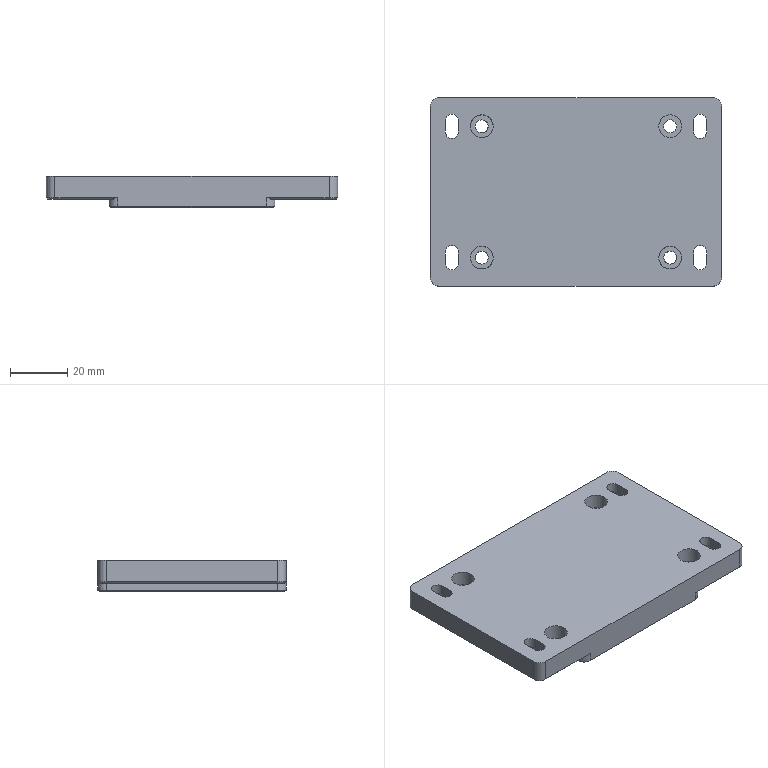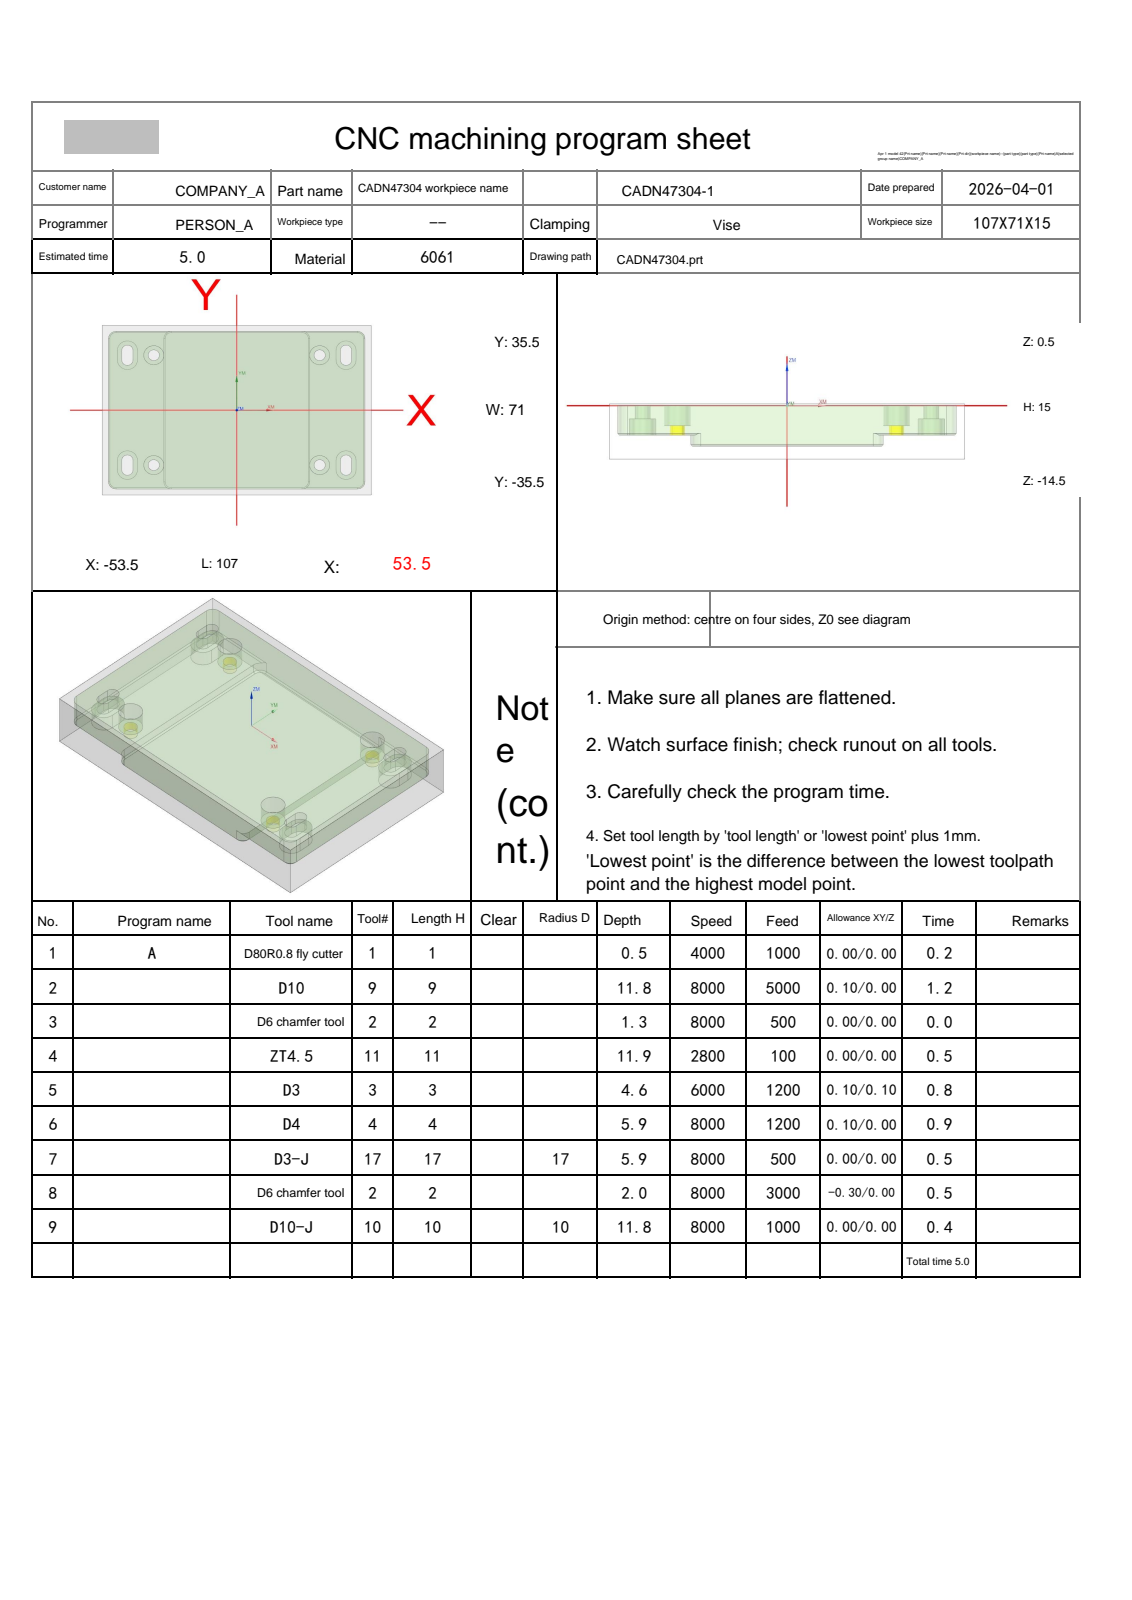NC program | NX | posted by the shop | part box 102 x 66 x 11 mm
Whole program:
%
O0001
(Machine time: 6.80 MIN)
(===Total Tool:8===)
(T1=D80R0.8 fly cutter D=80.  R=0.8  D-  H01 Z=-0.   )
(T9=D10     D=10.  R=0.   D-  H09 Z=-11.3 )
(T2=D6 chamfer tool   D=6.   R=0.   D-  H02 Z=-1.5  )
(T11=ZT4.5  D=4.5  DR_a=118 D-  H11 Z=-11.35)
(T3=D3      D=3.   R=0.   D-  H03 Z=-4.1  )
(T4=D4      D=4.   R=0.   D-  H04 Z=-5.4  )
(T17=D3-J   D=3.   R=0.   D17 H17 Z=-5.4  )
(T10=D10-J  D=10.  R=0.   D10 H10 Z=-11.3 )
G80 G90 G17 G49 G40
G91 G28 Z0
M01
N1 T01 M06
(D80R0.8 fly cutter  D=80. R=0.8 H=01 ce=0.00 di=0.00)
G00 G90 G54 X-96. Y0.0 M03 S4000
G43 H01 Z20.
M08
Z2.
G01 Z0.0 F1000.
X-91.
X91.
X96.
Z2.
G00 Z20.
G91 G28 Z0.0
M05
M09
G91 G28 Z0.0
M01
N2 T09 M06
(D10  D=10. R=0. H=09 ce=0.10 di=0.00)
G00 G90 G54 X0.0 Y38.1 M03 S8000
G43 H09 Z20.
M08
Z.5
G01 X48. Z.396 F5000.
G02 X56.1 Y30. Z.368 I0.0 J-8.1
G01 Y-30. Z.238
G02 X48. Y-38.1 Z.211 I-8.1 J0.0
G01 X-48. Z.003
G02 X-56.1 Y-30. Z-.025 I0.0 J8.1
G01 Y30. Z-.155
G02 X-48. Y38.1 Z-.183 I8.1 J0.0
G01 X48. Z-.391
G02 X56.1 Y30. Z-.418 I0.0 J-8.1
G01 Y-30. Z-.548
G02 X48. Y-38.1 Z-.576 I-8.1 J0.0
G01 X-48. Z-.784
G02 X-56.1 Y-30. Z-.812 I0.0 J8.1
G01 Y30. Z-.942
G02 X-48. Y38.1 Z-.969 I8.1 J0.0
G01 X48. Z-1.177
G02 X56.1 Y30. Z-1.205 I0.0 J-8.1
G01 Y-30. Z-1.335
G02 X48. Y-38.1 Z-1.363 I-8.1 J0.0
G01 X-48. Z-1.571
G02 X-56.1 Y-30. Z-1.598 I0.0 J8.1
G01 Y30. Z-1.728
G02 X-48. Y38.1 Z-1.756 I8.1 J0.0
G01 X48. Z-1.964
G02 X56.1 Y30. Z-1.992 I0.0 J-8.1
G01 Y-30. Z-2.122
G02 X48. Y-38.1 Z-2.149 I-8.1 J0.0
G01 X-48. Z-2.357
G02 X-56.1 Y-30. Z-2.385 I0.0 J8.1
G01 Y30. Z-2.515
G02 X-48. Y38.1 Z-2.543 I8.1 J0.0
G01 X48. Z-2.751
G02 X56.1 Y30. Z-2.778 I0.0 J-8.1
G01 Y-30. Z-2.908
G02 X48. Y-38.1 Z-2.936 I-8.1 J0.0
G01 X-48. Z-3.144
G02 X-56.1 Y-30. Z-3.172 I0.0 J8.1
G01 Y30. Z-3.302
G02 X-48. Y38.1 Z-3.329 I8.1 J0.0
G01 X48. Z-3.537
G02 X56.1 Y30. Z-3.565 I0.0 J-8.1
G01 Y-30. Z-3.695
G02 X48. Y-38.1 Z-3.723 I-8.1 J0.0
G01 X-48. Z-3.931
G02 X-56.1 Y-30. Z-3.958 I0.0 J8.1
G01 Y30. Z-4.088
G02 X-48. Y38.1 Z-4.116 I8.1 J0.0
G01 X48. Z-4.324
G02 X56.1 Y30. Z-4.352 I0.0 J-8.1
G01 Y-30. Z-4.482
G02 X48. Y-38.1 Z-4.509 I-8.1 J0.0
G01 X-48. Z-4.717
G02 X-56.1 Y-30. Z-4.745 I0.0 J8.1
G01 Y30. Z-4.875
G02 X-48. Y38.1 Z-4.903 I8.1 J0.0
G01 X48. Z-5.111
G02 X56.1 Y30. Z-5.138 I0.0 J-8.1
G01 Y-30. Z-5.268
G02 X48. Y-38.1 Z-5.296 I-8.1 J0.0
G01 X-48. Z-5.504
G02 X-56.1 Y-30. Z-5.532 I0.0 J8.1
G01 Y30. Z-5.662
G02 X-48. Y38.1 Z-5.689 I8.1 J0.0
G01 X48. Z-5.897
G02 X56.1 Y30. Z-5.925 I0.0 J-8.1
G01 Y-30. Z-6.055
G02 X48. Y-38.1 Z-6.083 I-8.1 J0.0
G01 X-48. Z-6.291
G02 X-56.1 Y-30. Z-6.318 I0.0 J8.1
G01 Y30. Z-6.448
G02 X-48. Y38.1 Z-6.476 I8.1 J0.0
G01 X48. Z-6.684
G02 X56.1 Y30. Z-6.712 I0.0 J-8.1
G01 Y-30. Z-6.842
G02 X48. Y-38.1 Z-6.869 I-8.1 J0.0
G01 X-48. Z-7.077
G02 X-56.1 Y-30. Z-7.105 I0.0 J8.1
G01 Y30. Z-7.235
G02 X-48. Y38.1 Z-7.263 I8.1 J0.0
G01 X48. Z-7.471
G02 X56.1 Y30. Z-7.498 I0.0 J-8.1
G01 Y-30. Z-7.628
G02 X48. Y-38.1 Z-7.656 I-8.1 J0.0
G01 X-48. Z-7.864
G02 X-56.1 Y-30. Z-7.892 I0.0 J8.1
G01 Y30. Z-8.022
G02 X-48. Y38.1 Z-8.049 I8.1 J0.0
G01 X48. Z-8.257
G02 X56.1 Y30. Z-8.285 I0.0 J-8.1
G01 Y-30. Z-8.415
G02 X48. Y-38.1 Z-8.443 I-8.1 J0.0
G01 X-48. Z-8.651
G02 X-56.1 Y-30. Z-8.678 I0.0 J8.1
G01 Y30. Z-8.808
G02 X-48. Y38.1 Z-8.836 I8.1 J0.0
G01 X48. Z-9.044
G02 X56.1 Y30. Z-9.072 I0.0 J-8.1
G01 Y-30. Z-9.202
G02 X48. Y-38.1 Z-9.229 I-8.1 J0.0
G01 X-48. Z-9.437
G02 X-56.1 Y-30. Z-9.465 I0.0 J8.1
G01 Y30. Z-9.595
G02 X-48. Y38.1 Z-9.623 I8.1 J0.0
G01 X48. Z-9.831
G02 X56.1 Y30. Z-9.858 I0.0 J-8.1
G01 Y-30. Z-9.988
G02 X48. Y-38.1 Z-10.016 I-8.1 J0.0
G01 X-48. Z-10.224
G02 X-56.1 Y-30. Z-10.252 I0.0 J8.1
G01 Y30. Z-10.382
G02 X-48. Y38.1 Z-10.409 I8.1 J0.0
G01 X48. Z-10.617
G02 X56.1 Y30. Z-10.645 I0.0 J-8.1
G01 Y-30. Z-10.775
G02 X48. Y-38.1 Z-10.803 I-8.1 J0.0
G01 X-48. Z-11.011
G02 X-56.1 Y-30. Z-11.038 I0.0 J8.1
G01 Y30. Z-11.168
G02 X-48. Y38.1 Z-11.196 I8.1 J0.0
G01 X0.0 Z-11.3
X48.
G02 X56.1 Y30. I0.0 J-8.1
G01 Y-30.
G02 X48. Y-38.1 I-8.1 J0.0
G01 X-48.
G02 X-56.1 Y-30. I0.0 J8.1
G01 Y30.
G02 X-48. Y38.1 I8.1 J0.0
G01 X0.0
X.5
Z-10.3
G00 Z20.
G91 G28 Z0.0
M05
M09
G91 G28 Z0.0
M01
N3 T02 M06
(D6 chamfer tool  D=6. R=0. H=02 ce=0.00 di=0.00)
G00 G90 G54 X-33. Y23. M03 S8000
G43 H02 Z20.
M08
G98 G81 X-33. Y23. Z-.8 R1. F500.
Y-23.
X33.
Y23.
G80
G00 Z20.
G91 G28 Z0.0
M05
M09
G91 G28 Z0.0
M01
N4 T11 M06
(ZT4.5 D=4.5 DR_a=118 H=11)
G00 G90 G54 X-33. Y23. M03 S2800
G43 H11 Z20.
M08
G98 G83 X-33. Y23. Z-11.352 R1. F100. Q2.
Y-23.
X33.
Y23.
G80
G00 Z20.
G91 G28 Z0.0
M05
M09
G91 G28 Z0.0
M01
N5 T03 M06
(D3  D=3. R=0. H=03 ce=0.10 di=0.10)
G00 G90 G54 X-44.15 Y-23. M03 S6000
G43 H03 Z20.
M08
Z.5
G01 Y-25. Z.46 F1200.
G03 X-43.5 Y-25.65 Z.439 I.65 J0.0
X-42.85 Y-25. Z.419 I0.0 J.65
G01 Y-21. Z.339
G03 X-43.5 Y-20.35 Z.318 I-.65 J0.0
X-44.015 Y-20.603 Z.307 I0.0 J-.65
X-44.15 Y-21. Z.298 I.515 J-.397
G01 Y-25. Z.218
G03 X-43.5 Y-25.65 Z.197 I.65 J0.0
X-42.85 Y-25. Z.177 I0.0 J.65
G01 Y-21. Z.097
G03 X-43.5 Y-20.35 Z.076 I-.65 J0.0
X-44.015 Y-20.603 Z.064 I0.0 J-.65
X-44.15 Y-21. Z.056 I.515 J-.397
G01 Y-25. Z-.024
G03 X-43.5 Y-25.65 Z-.045 I.65 J0.0
X-42.85 Y-25. Z-.065 I0.0 J.65
G01 Y-21. Z-.145
G03 X-43.5 Y-20.35 Z-.166 I-.65 J0.0
X-44.015 Y-20.603 Z-.178 I0.0 J-.65
X-44.15 Y-21. Z-.186 I.515 J-.397
G01 Y-25. Z-.266
G03 X-43.5 Y-25.65 Z-.287 I.65 J0.0
X-42.85 Y-25. Z-.307 I0.0 J.65
G01 Y-21. Z-.387
G03 X-43.5 Y-20.35 Z-.408 I-.65 J0.0
X-44.015 Y-20.603 Z-.42 I0.0 J-.65
X-44.15 Y-21. Z-.428 I.515 J-.397
G01 Y-25. Z-.508
G03 X-43.5 Y-25.65 Z-.529 I.65 J0.0
X-42.85 Y-25. Z-.549 I0.0 J.65
G01 Y-21. Z-.63
G03 X-43.5 Y-20.35 Z-.65 I-.65 J0.0
X-44.015 Y-20.603 Z-.662 I0.0 J-.65
X-44.15 Y-21. Z-.67 I.515 J-.397
G01 Y-25. Z-.751
G03 X-43.5 Y-25.65 Z-.771 I.65 J0.0
X-42.85 Y-25. Z-.792 I0.0 J.65
G01 Y-21. Z-.872
G03 X-43.5 Y-20.35 Z-.892 I-.65 J0.0
X-44.015 Y-20.603 Z-.904 I0.0 J-.65
X-44.15 Y-21. Z-.913 I.515 J-.397
G01 Y-25. Z-.993
G03 X-43.5 Y-25.65 Z-1.013 I.65 J0.0
X-42.85 Y-25. Z-1.034 I0.0 J.65
G01 Y-21. Z-1.114
G03 X-43.5 Y-20.35 Z-1.134 I-.65 J0.0
X-44.015 Y-20.603 Z-1.146 I0.0 J-.65
X-44.15 Y-21. Z-1.155 I.515 J-.397
G01 Y-25. Z-1.235
G03 X-43.5 Y-25.65 Z-1.255 I.65 J0.0
X-42.85 Y-25. Z-1.276 I0.0 J.65
G01 Y-21. Z-1.356
G03 X-43.5 Y-20.35 Z-1.376 I-.65 J0.0
X-44.015 Y-20.603 Z-1.388 I0.0 J-.65
X-44.15 Y-21. Z-1.397 I.515 J-.397
G01 Y-25. Z-1.477
G03 X-43.5 Y-25.65 Z-1.497 I.65 J0.0
X-42.85 Y-25. Z-1.518 I0.0 J.65
G01 Y-21. Z-1.598
G03 X-43.5 Y-20.35 Z-1.618 I-.65 J0.0
X-44.015 Y-20.603 Z-1.63 I0.0 J-.65
X-44.15 Y-21. Z-1.639 I.515 J-.397
G01 Y-25. Z-1.719
G03 X-43.5 Y-25.65 Z-1.739 I.65 J0.0
X-42.85 Y-25. Z-1.76 I0.0 J.65
G01 Y-21. Z-1.84
G03 X-43.5 Y-20.35 Z-1.861 I-.65 J0.0
X-44.015 Y-20.603 Z-1.872 I0.0 J-.65
X-44.15 Y-21. Z-1.881 I.515 J-.397
G01 Y-25. Z-1.961
G03 X-43.5 Y-25.65 Z-1.982 I.65 J0.0
X-42.85 Y-25. Z-2.002 I0.0 J.65
G01 Y-21. Z-2.082
G03 X-43.5 Y-20.35 Z-2.103 I-.65 J0.0
X-44.015 Y-20.603 Z-2.115 I0.0 J-.65
X-44.15 Y-21. Z-2.123 I.515 J-.397
G01 Y-25. Z-2.203
G03 X-43.5 Y-25.65 Z-2.224 I.65 J0.0
X-42.85 Y-25. Z-2.244 I0.0 J.65
G01 Y-21. Z-2.324
G03 X-43.5 Y-20.35 Z-2.345 I-.65 J0.0
X-44.015 Y-20.603 Z-2.357 I0.0 J-.65
X-44.15 Y-21. Z-2.365 I.515 J-.397
G01 Y-25. Z-2.445
G03 X-43.5 Y-25.65 Z-2.466 I.65 J0.0
X-42.85 Y-25. Z-2.486 I0.0 J.65
G01 Y-21. Z-2.566
G03 X-43.5 Y-20.35 Z-2.587 I-.65 J0.0
X-44.015 Y-20.603 Z-2.599 I0.0 J-.65
X-44.15 Y-21. Z-2.607 I.515 J-.397
G01 Y-25. Z-2.687
G03 X-43.5 Y-25.65 Z-2.708 I.65 J0.0
X-42.85 Y-25. Z-2.728 I0.0 J.65
G01 Y-21. Z-2.808
G03 X-43.5 Y-20.35 Z-2.829 I-.65 J0.0
X-44.015 Y-20.603 Z-2.841 I0.0 J-.65
X-44.15 Y-21. Z-2.849 I.515 J-.397
G01 Y-25. Z-2.93
G03 X-43.5 Y-25.65 Z-2.95 I.65 J0.0
X-42.85 Y-25. Z-2.97 I0.0 J.65
G01 Y-21. Z-3.051
G03 X-43.5 Y-20.35 Z-3.071 I-.65 J0.0
X-44.015 Y-20.603 Z-3.083 I0.0 J-.65
X-44.15 Y-21. Z-3.092 I.515 J-.397
G01 Y-25. Z-3.172
G03 X-43.5 Y-25.65 Z-3.192 I.65 J0.0
X-42.85 Y-25. Z-3.213 I0.0 J.65
G01 Y-21. Z-3.293
G03 X-43.5 Y-20.35 Z-3.313 I-.65 J0.0
X-44.015 Y-20.603 Z-3.325 I0.0 J-.65
X-44.15 Y-21. Z-3.334 I.515 J-.397
G01 Y-25. Z-3.414
G03 X-43.5 Y-25.65 Z-3.434 I.65 J0.0
X-42.85 Y-25. Z-3.455 I0.0 J.65
G01 Y-21. Z-3.535
G03 X-43.5 Y-20.35 Z-3.555 I-.65 J0.0
X-44.015 Y-20.603 Z-3.567 I0.0 J-.65
X-44.15 Y-21. Z-3.576 I.515 J-.397
G01 Y-25. Z-3.656
G03 X-43.5 Y-25.65 Z-3.676 I.65 J0.0
X-42.85 Y-25. Z-3.697 I0.0 J.65
G01 Y-21. Z-3.777
G03 X-43.5 Y-20.35 Z-3.797 I-.65 J0.0
X-44.015 Y-20.603 Z-3.809 I0.0 J-.65
X-44.15 Y-21. Z-3.818 I.515 J-.397
G01 Y-25. Z-3.898
G03 X-43.5 Y-25.65 Z-3.918 I.65 J0.0
X-42.85 Y-25. Z-3.939 I0.0 J.65
G01 Y-21. Z-4.019
G03 X-43.5 Y-20.35 Z-4.039 I-.65 J0.0
X-44.015 Y-20.603 Z-4.051 I0.0 J-.65
X-44.15 Y-21. Z-4.06 I.515 J-.397
G01 Y-23. Z-4.1
Y-25.
G03 X-43.5 Y-25.65 I.65 J0.0
X-42.85 Y-25. I0.0 J.65
G01 Y-21.
G03 X-43.5 Y-20.35 I-.65 J0.0
X-44.15 Y-21. I0.0 J-.65
G01 Y-23.
Y-23.5
Z-3.1
G00 Z20.
Y23.
Z.5
G01 Y21. Z.46
G03 X-43.5 Y20.35 Z.439 I.65 J0.0
X-42.85 Y21. Z.419 I0.0 J.65
G01 Y25. Z.339
G03 X-43.5 Y25.65 Z.318 I-.65 J0.0
X-44.15 Y25. Z.298 I0.0 J-.65
G01 Y21. Z.218
G03 X-43.5 Y20.35 Z.197 I.65 J0.0
X-42.85 Y21. Z.177 I0.0 J.65
G01 Y25. Z.097
G03 X-43.5 Y25.65 Z.076 I-.65 J0.0
X-44.15 Y25. Z.056 I0.0 J-.65
G01 Y21. Z-.024
G03 X-43.5 Y20.35 Z-.045 I.65 J0.0
X-42.85 Y21. Z-.065 I0.0 J.65
G01 Y25. Z-.145
G03 X-43.5 Y25.65 Z-.166 I-.65 J0.0
X-44.15 Y25. Z-.186 I0.0 J-.65
G01 Y21. Z-.266
G03 X-43.5 Y20.35 Z-.287 I.65 J0.0
X-42.85 Y21. Z-.307 I0.0 J.65
G01 Y25. Z-.387
G03 X-43.5 Y25.65 Z-.408 I-.65 J0.0
X-44.15 Y25. Z-.428 I0.0 J-.65
G01 Y21. Z-.508
G03 X-43.5 Y20.35 Z-.529 I.65 J0.0
X-42.85 Y21. Z-.549 I0.0 J.65
G01 Y25. Z-.63
G03 X-43.5 Y25.65 Z-.65 I-.65 J0.0
X-44.15 Y25. Z-.67 I0.0 J-.65
G01 Y21. Z-.751
G03 X-43.5 Y20.35 Z-.771 I.65 J0.0
X-42.85 Y21. Z-.792 I0.0 J.65
G01 Y25. Z-.872
G03 X-43.5 Y25.65 Z-.892 I-.65 J0.0
X-44.15 Y25. Z-.913 I0.0 J-.65
G01 Y21. Z-.993
G03 X-43.5 Y20.35 Z-1.013 I.65 J0.0
X-42.85 Y21. Z-1.034 I0.0 J.65
G01 Y25. Z-1.114
G03 X-43.5 Y25.65 Z-1.134 I-.65 J0.0
X-44.15 Y25. Z-1.155 I0.0 J-.65
G01 Y21. Z-1.235
G03 X-43.5 Y20.35 Z-1.255 I.65 J0.0
X-42.85 Y21. Z-1.276 I0.0 J.65
G01 Y25. Z-1.356
G03 X-43.5 Y25.65 Z-1.376 I-.65 J0.0
X-44.15 Y25. Z-1.397 I0.0 J-.65
G01 Y21. Z-1.477
G03 X-43.5 Y20.35 Z-1.497 I.65 J0.0
X-42.85 Y21. Z-1.518 I0.0 J.65
G01 Y25. Z-1.598
G03 X-43.5 Y25.65 Z-1.618 I-.65 J0.0
X-44.15 Y25. Z-1.639 I0.0 J-.65
G01 Y21. Z-1.719
G03 X-43.5 Y20.35 Z-1.739 I.65 J0.0
X-42.85 Y21. Z-1.76 I0.0 J.65
G01 Y25. Z-1.84
G03 X-43.5 Y25.65 Z-1.861 I-.65 J0.0
X-44.15 Y25. Z-1.881 I0.0 J-.65
G01 Y21. Z-1.961
G03 X-43.5 Y20.35 Z-1.982 I.65 J0.0
X-42.85 Y21. Z-2.002 I0.0 J.65
G01 Y25. Z-2.082
G03 X-43.5 Y25.65 Z-2.103 I-.65 J0.0
X-44.15 Y25. Z-2.123 I0.0 J-.65
G01 Y21. Z-2.203
G03 X-43.5 Y20.35 Z-2.224 I.65 J0.0
X-42.85 Y21. Z-2.244 I0.0 J.65
G01 Y25. Z-2.324
G03 X-43.5 Y25.65 Z-2.345 I-.65 J0.0
X-44.15 Y25. Z-2.365 I0.0 J-.65
G01 Y21. Z-2.445
G03 X-43.5 Y20.35 Z-2.466 I.65 J0.0
X-42.85 Y21. Z-2.486 I0.0 J.65
G01 Y25. Z-2.566
G03 X-43.5 Y25.65 Z-2.587 I-.65 J0.0
X-44.15 Y25. Z-2.607 I0.0 J-.65
G01 Y21. Z-2.687
G03 X-43.5 Y20.35 Z-2.708 I.65 J0.0
X-42.85 Y21. Z-2.728 I0.0 J.65
G01 Y25. Z-2.808
G03 X-43.5 Y25.65 Z-2.829 I-.65 J0.0
X-44.15 Y25. Z-2.849 I0.0 J-.65
G01 Y21. Z-2.93
G03 X-43.5 Y20.35 Z-2.95 I.65 J0.0
X-42.85 Y21. Z-2.97 I0.0 J.65
G01 Y25. Z-3.051
G03 X-43.5 Y25.65 Z-3.071 I-.65 J0.0
X-44.15 Y25. Z-3.092 I0.0 J-.65
G01 Y21. Z-3.172
G03 X-43.5 Y20.35 Z-3.192 I.65 J0.0
X-42.85 Y21. Z-3.213 I0.0 J.65
G01 Y25. Z-3.293
G03 X-43.5 Y25.65 Z-3.313 I-.65 J0.0
X-44.15 Y25. Z-3.334 I0.0 J-.65
G01 Y21. Z-3.414
G03 X-43.5 Y20.35 Z-3.434 I.65 J0.0
X-42.85 Y21. Z-3.455 I0.0 J.65
G01 Y25. Z-3.535
G03 X-43.5 Y25.65 Z-3.555 I-.65 J0.0
X-44.15 Y25. Z-3.576 I0.0 J-.65
G01 Y21. Z-3.656
G03 X-43.5 Y20.35 Z-3.676 I.65 J0.0
X-42.85 Y21. Z-3.697 I0.0 J.65
G01 Y25. Z-3.777
G03 X-43.5 Y25.65 Z-3.797 I-.65 J0.0
X-44.15 Y25. Z-3.818 I0.0 J-.65
G01 Y21. Z-3.898
G03 X-43.5 Y20.35 Z-3.918 I.65 J0.0
X-42.85 Y21. Z-3.939 I0.0 J.65
G01 Y25. Z-4.019
G03 X-43.5 Y25.65 Z-4.039 I-.65 J0.0
X-44.15 Y25. Z-4.06 I0.0 J-.65
G01 Y23. Z-4.1
Y21.
G03 X-43.5 Y20.35 I.65 J0.0
X-42.85 Y21. I0.0 J.65
G01 Y25.
G03 X-43.5 Y25.65 I-.65 J0.0
X-44.15 Y25. I0.0 J-.65
G01 Y23.
Y22.5
Z-3.1
G00 Z20.
X44.15 Y23.
Z.5
G01 Y25. Z.46
G03 X43.5 Y25.65 Z.439 I-.65 J0.0
X42.85 Y25. Z.419 I0.0 J-.65
G01 Y21. Z.339
G03 X43.5 Y20.35 Z.318 I.65 J0.0
X44.15 Y21. Z.298 I0.0 J.65
G01 Y25. Z.218
G03 X43.5 Y25.65 Z.197 I-.65 J0.0
X42.85 Y25. Z.177 I0.0 J-.65
G01 Y21. Z.097
G03 X43.5 Y20.35 Z.076 I.65 J0.0
X44.15 Y21. Z.056 I0.0 J.65
G01 Y25. Z-.024
G03 X43.5 Y25.65 Z-.045 I-.65 J0.0
X42.85 Y25. Z-.065 I0.0 J-.65
G01 Y21. Z-.145
G03 X43.5 Y20.35 Z-.166 I.65 J0.0
X44.15 Y21. Z-.186 I0.0 J.65
G01 Y25. Z-.266
G03 X43.5 Y25.65 Z-.287 I-.65 J0.0
X42.85 Y25. Z-.307 I0.0 J-.65
G01 Y21. Z-.387
G03 X43.5 Y20.35 Z-.408 I.65 J0.0
X44.15 Y21. Z-.428 I0.0 J.65
G01 Y25. Z-.508
G03 X43.5 Y25.65 Z-.529 I-.65 J0.0
X42.85 Y25. Z-.549 I0.0 J-.65
G01 Y21. Z-.63
G03 X43.5 Y20.35 Z-.65 I.65 J0.0
X44.15 Y21. Z-.67 I0.0 J.65
G01 Y25. Z-.751
G03 X43.5 Y25.65 Z-.771 I-.65 J0.0
X42.85 Y25. Z-.792 I0.0 J-.65
G01 Y21. Z-.872
G03 X43.5 Y20.35 Z-.892 I.65 J0.0
X44.15 Y21. Z-.913 I0.0 J.65
G01 Y25. Z-.993
G03 X43.5 Y25.65 Z-1.013 I-.65 J0.0
X42.85 Y25. Z-1.034 I0.0 J-.65
G01 Y21. Z-1.114
G03 X43.5 Y20.35 Z-1.134 I.65 J0.0
X44.15 Y21. Z-1.155 I0.0 J.65
G01 Y25. Z-1.235
G03 X43.5 Y25.65 Z-1.255 I-.65 J0.0
X42.85 Y25. Z-1.276 I0.0 J-.65
G01 Y21. Z-1.356
G03 X43.5 Y20.35 Z-1.376 I.65 J0.0
X44.15 Y21. Z-1.397 I0.0 J.65
G01 Y25. Z-1.477
G03 X43.5 Y25.65 Z-1.497 I-.65 J0.0
X42.85 Y25. Z-1.518 I0.0 J-.65
G01 Y21. Z-1.598
G03 X43.5 Y20.35 Z-1.618 I.65 J0.0
X44.15 Y21. Z-1.639 I0.0 J.65
G01 Y25. Z-1.719
G03 X43.5 Y25.65 Z-1.739 I-.65 J0.0
X42.85 Y25. Z-1.76 I0.0 J-.65
G01 Y21. Z-1.84
G03 X43.5 Y20.35 Z-1.861 I.65 J0.0
X44.15 Y21. Z-1.881 I0.0 J.65
G01 Y25. Z-1.961
G03 X43.5 Y25.65 Z-1.982 I-.65 J0.0
X42.85 Y25. Z-2.002 I0.0 J-.65
G01 Y21. Z-2.082
G03 X43.5 Y20.35 Z-2.103 I.65 J0.0
X44.15 Y21. Z-2.123 I0.0 J.65
G01 Y25. Z-2.203
G03 X43.5 Y25.65 Z-2.224 I-.65 J0.0
X42.85 Y25. Z-2.244 I0.0 J-.65
G01 Y21. Z-2.324
G03 X43.5 Y20.35 Z-2.345 I.65 J0.0
X44.15 Y21. Z-2.365 I0.0 J.65
G01 Y25. Z-2.445
G03 X43.5 Y25.65 Z-2.466 I-.65 J0.0
X42.85 Y25. Z-2.486 I0.0 J-.65
G01 Y21. Z-2.566
G03 X43.5 Y20.35 Z-2.587 I.65 J0.0
X44.15 Y21. Z-2.607 I0.0 J.65
G01 Y25. Z-2.687
G03 X43.5 Y25.65 Z-2.708 I-.65 J0.0
X42.85 Y25. Z-2.728 I0.0 J-.65
G01 Y21. Z-2.808
G03 X43.5 Y20.35 Z-2.829 I.65 J0.0
X44.15 Y21. Z-2.849 I0.0 J.65
G01 Y25. Z-2.93
G03 X43.5 Y25.65 Z-2.95 I-.65 J0.0
X42.85 Y25. Z-2.97 I0.0 J-.65
G01 Y21. Z-3.051
G03 X43.5 Y20.35 Z-3.071 I.65 J0.0
X44.15 Y21. Z-3.092 I0.0 J.65
G01 Y25. Z-3.172
G03 X43.5 Y25.65 Z-3.192 I-.65 J0.0
X42.85 Y25. Z-3.213 I0.0 J-.65
G01 Y21. Z-3.293
G03 X43.5 Y20.35 Z-3.313 I.65 J0.0
X44.15 Y21. Z-3.334 I0.0 J.65
G01 Y25. Z-3.414
G03 X43.5 Y25.65 Z-3.434 I-.65 J0.0
X42.85 Y25. Z-3.455 I0.0 J-.65
G01 Y21. Z-3.535
G03 X43.5 Y20.35 Z-3.555 I.65 J0.0
X44.15 Y21. Z-3.576 I0.0 J.65
G01 Y25. Z-3.656
G03 X43.5 Y25.65 Z-3.676 I-.65 J0.0
X42.85 Y25. Z-3.697 I0.0 J-.65
G01 Y21. Z-3.777
G03 X43.5 Y20.35 Z-3.797 I.65 J0.0
X44.15 Y21. Z-3.818 I0.0 J.65
G01 Y25. Z-3.898
G03 X43.5 Y25.65 Z-3.918 I-.65 J0.0
X42.85 Y25. Z-3.939 I0.0 J-.65
G01 Y21. Z-4.019
G03 X43.5 Y20.35 Z-4.039 I.65 J0.0
X44.15 Y21. Z-4.06 I0.0 J.65
G01 Y23. Z-4.1
Y25.
G03 X43.5 Y25.65 I-.65 J0.0
X42.85 Y25. I0.0 J-.65
G01 Y21.
G03 X43.5 Y20.35 I.65 J0.0
X44.15 Y21. I0.0 J.65
G01 Y23.
Y23.5
Z-3.1
G00 Z20.
Y-23.
Z.5
G01 Y-21. Z.46
G03 X43.5 Y-20.35 Z.439 I-.65 J0.0
X42.85 Y-21. Z.419 I0.0 J-.65
G01 Y-25. Z.339
G03 X43.5 Y-25.65 Z.318 I.65 J0.0
X44.15 Y-25. Z.298 I0.0 J.65
G01 Y-21. Z.218
G03 X43.5 Y-20.35 Z.197 I-.65 J0.0
X42.85 Y-21. Z.177 I0.0 J-.65
G01 Y-25. Z.097
G03 X43.5 Y-25.65 Z.076 I.65 J0.0
X44.15 Y-25. Z.056 I0.0 J.65
G01 Y-21. Z-.024
G03 X43.5 Y-20.35 Z-.045 I-.65 J0.0
X42.85 Y-21. Z-.065 I0.0 J-.65
G01 Y-25. Z-.145
G03 X43.5 Y-25.65 Z-.166 I.65 J0.0
X44.15 Y-25. Z-.186 I0.0 J.65
G01 Y-21. Z-.266
G03 X43.5 Y-20.35 Z-.287 I-.65 J0.0
X42.85 Y-21. Z-.307 I0.0 J-.65
G01 Y-25. Z-.387
G03 X43.5 Y-25.65 Z-.408 I.65 J0.0
X44.15 Y-25. Z-.428 I0.0 J.65
G01 Y-21. Z-.508
G03 X43.5 Y-20.35 Z-.529 I-.65 J0.0
X42.85 Y-21. Z-.549 I0.0 J-.65
G01 Y-25. Z-.63
G03 X43.5 Y-25.65 Z-.65 I.65 J0.0
X44.15 Y-25. Z-.67 I0.0 J.65
G01 Y-21. Z-.751
G03 X43.5 Y-20.35 Z-.771 I-.65 J0.0
X42.85 Y-21. Z-.792 I0.0 J-.65
G01 Y-25. Z-.872
G03 X43.5 Y-25.65 Z-.892 I.65 J0.0
X44.15 Y-25. Z-.913 I0.0 J.65
G01 Y-21. Z-.993
G03 X43.5 Y-20.35 Z-1.013 I-.65 J0.0
X42.85 Y-21. Z-1.034 I0.0 J-.65
G01 Y-25. Z-1.114
G03 X43.5 Y-25.65 Z-1.134 I.65 J0.0
X44.15 Y-25. Z-1.155 I0.0 J.65
G01 Y-21. Z-1.235
G03 X43.5 Y-20.35 Z-1.255 I-.65 J0.0
X42.85 Y-21. Z-1.276 I0.0 J-.65
G01 Y-25. Z-1.356
G03 X43.5 Y-25.65 Z-1.376 I.65 J0.0
X44.15 Y-25. Z-1.397 I0.0 J.65
G01 Y-21. Z-1.477
G03 X43.5 Y-20.35 Z-1.497 I-.65 J0.0
X42.85 Y-21. Z-1.518 I0.0 J-.65
G01 Y-25. Z-1.598
G03 X43.5 Y-25.65 Z-1.618 I.65 J0.0
X44.15 Y-25. Z-1.639 I0.0 J.65
G01 Y-21. Z-1.719
G03 X43.5 Y-20.35 Z-1.739 I-.65 J0.0
X42.85 Y-21. Z-1.76 I0.0 J-.65
G01 Y-25. Z-1.84
G03 X43.5 Y-25.65 Z-1.861 I.65 J0.0
X44.15 Y-25. Z-1.881 I0.0 J.65
G01 Y-21. Z-1.961
G03 X43.5 Y-20.35 Z-1.982 I-.65 J0.0
X42.85 Y-21. Z-2.002 I0.0 J-.65
G01 Y-25. Z-2.082
G03 X43.5 Y-25.65 Z-2.103 I.65 J0.0
X44.15 Y-25. Z-2.123 I0.0 J.65
G01 Y-21. Z-2.203
G03 X43.5 Y-20.35 Z-2.224 I-.65 J0.0
X42.85 Y-21. Z-2.244 I0.0 J-.65
G01 Y-25. Z-2.324
G03 X43.5 Y-25.65 Z-2.345 I.65 J0.0
X44.15 Y-25. Z-2.365 I0.0 J.65
G01 Y-21. Z-2.445
G03 X43.5 Y-20.35 Z-2.466 I-.65 J0.0
X42.85 Y-21. Z-2.486 I0.0 J-.65
G01 Y-25. Z-2.566
G03 X43.5 Y-25.65 Z-2.587 I.65 J0.0
X44.15 Y-25. Z-2.607 I0.0 J.65
G01 Y-21. Z-2.687
G03 X43.5 Y-20.35 Z-2.708 I-.65 J0.0
X42.85 Y-21. Z-2.728 I0.0 J-.65
G01 Y-25. Z-2.808
G03 X43.5 Y-25.65 Z-2.829 I.65 J0.0
X44.15 Y-25. Z-2.849 I0.0 J.65
G01 Y-21. Z-2.93
G03 X43.5 Y-20.35 Z-2.95 I-.65 J0.0
X42.85 Y-21. Z-2.97 I0.0 J-.65
G01 Y-25. Z-3.051
G03 X43.5 Y-25.65 Z-3.071 I.65 J0.0
X44.15 Y-25. Z-3.092 I0.0 J.65
G01 Y-21. Z-3.172
G03 X43.5 Y-20.35 Z-3.192 I-.65 J0.0
X42.85 Y-21. Z-3.213 I0.0 J-.65
G01 Y-25. Z-3.293
G03 X43.5 Y-25.65 Z-3.313 I.65 J0.0
X44.15 Y-25. Z-3.334 I0.0 J.65
G01 Y-21. Z-3.414
G03 X43.5 Y-20.35 Z-3.434 I-.65 J0.0
X42.85 Y-21. Z-3.455 I0.0 J-.65
G01 Y-25. Z-3.535
G03 X43.5 Y-25.65 Z-3.555 I.65 J0.0
X44.15 Y-25. Z-3.576 I0.0 J.65
G01 Y-21. Z-3.656
G03 X43.5 Y-20.35 Z-3.676 I-.65 J0.0
X42.85 Y-21. Z-3.697 I0.0 J-.65
G01 Y-25. Z-3.777
G03 X43.5 Y-25.65 Z-3.797 I.65 J0.0
X44.15 Y-25. Z-3.818 I0.0 J.65
G01 Y-21. Z-3.898
G03 X43.5 Y-20.35 Z-3.918 I-.65 J0.0
X42.85 Y-21. Z-3.939 I0.0 J-.65
G01 Y-25. Z-4.019
G03 X43.5 Y-25.65 Z-4.039 I.65 J0.0
X44.15 Y-25. Z-4.06 I0.0 J.65
G01 Y-23. Z-4.1
Y-21.
G03 X43.5 Y-20.35 I-.65 J0.0
X42.85 Y-21. I0.0 J-.65
G01 Y-25.
G03 X43.5 Y-25.65 I.65 J0.0
X44.15 Y-25. I0.0 J.65
G01 Y-23.
Y-22.5
Z-3.1
G00 Z20.
G91 G28 Z0.0
M05
M09
G91 G28 Z0.0
M01
N6 T04 M06
(D4  D=4. R=0. H=04 ce=0.10 di=0.00)
G00 G90 G54 X-33. Y23. M03 S8000
G43 H04 Z20.
M08
Z.5
G03 X-32.05 Y22.05 I.95 J0.0 F1200.
X-31.1 Y23. I0.0 J.95
X-31.1 Y23. Z.2 I-1.9 J0.0
X-31.1 Y23. Z-.1 I-1.9 J0.0
X-31.1 Y23. Z-.4 I-1.9 J0.0
X-31.1 Y23. Z-.7 I-1.9 J0.0
X-31.1 Y23. Z-1. I-1.9 J0.0
X-31.1 Y23. Z-1.3 I-1.9 J0.0
X-31.1 Y23. Z-1.6 I-1.9 J0.0
X-31.1 Y23. Z-1.9 I-1.9 J0.0
X-31.1 Y23. Z-2.2 I-1.9 J0.0
X-31.1 Y23. Z-2.5 I-1.9 J0.0
X-31.1 Y23. Z-2.8 I-1.9 J0.0
X-31.1 Y23. Z-3.1 I-1.9 J0.0
X-31.1 Y23. Z-3.4 I-1.9 J0.0
X-31.1 Y23. Z-3.7 I-1.9 J0.0
X-31.1 Y23. Z-4. I-1.9 J0.0
X-31.1 Y23. Z-4.3 I-1.9 J0.0
X-31.1 Y23. Z-4.6 I-1.9 J0.0
X-31.1 Y23. Z-4.9 I-1.9 J0.0
X-31.1 Y23. Z-5.2 I-1.9 J0.0
X-33.95 Y21.355 Z-5.4 I-1.9 J0.0
X-33. Y21.1 I.95 J1.645
X-31.1 Y23. I0.0 J1.9
X-33. Y24.9 I-1.9 J0.0
X-34.9 Y23. I0.0 J-1.9
X-33.95 Y21.355 I1.9 J0.0
X-33.475 Y21.227 I.475 J.823
X-32.525 Y22.177 I0.0 J.95
X-33. Y23. I-.95 J0.0
G00 Z20.
Y-23.
Z.5
G03 X-32.05 Y-23.95 I.95 J0.0
X-31.1 Y-23. I0.0 J.95
X-31.1 Y-23. Z.2 I-1.9 J0.0
X-31.1 Y-23. Z-.1 I-1.9 J0.0
X-31.1 Y-23. Z-.4 I-1.9 J0.0
X-31.1 Y-23. Z-.7 I-1.9 J0.0
X-31.1 Y-23. Z-1. I-1.9 J0.0
X-31.1 Y-23. Z-1.3 I-1.9 J0.0
X-31.1 Y-23. Z-1.6 I-1.9 J0.0
X-31.1 Y-23. Z-1.9 I-1.9 J0.0
X-31.1 Y-23. Z-2.2 I-1.9 J0.0
X-31.1 Y-23. Z-2.5 I-1.9 J0.0
X-31.1 Y-23. Z-2.8 I-1.9 J0.0
X-31.1 Y-23. Z-3.1 I-1.9 J0.0
X-31.1 Y-23. Z-3.4 I-1.9 J0.0
X-31.1 Y-23. Z-3.7 I-1.9 J0.0
X-31.1 Y-23. Z-4. I-1.9 J0.0
X-31.1 Y-23. Z-4.3 I-1.9 J0.0
X-31.1 Y-23. Z-4.6 I-1.9 J0.0
X-31.1 Y-23. Z-4.9 I-1.9 J0.0
X-31.1 Y-23. Z-5.2 I-1.9 J0.0
X-33.95 Y-24.645 Z-5.4 I-1.9 J0.0
X-33. Y-24.9 I.95 J1.645
X-31.1 Y-23. I0.0 J1.9
X-33. Y-21.1 I-1.9 J0.0
X-34.9 Y-23. I0.0 J-1.9
X-33.95 Y-24.645 I1.9 J0.0
X-33.475 Y-24.773 I.475 J.823
X-32.525 Y-23.823 I0.0 J.95
X-33. Y-23. I-.95 J0.0
G00 Z20.
X33.
Z.5
G03 X33.95 Y-23.95 I.95 J0.0
X34.9 Y-23. I0.0 J.95
X34.9 Y-23. Z.2 I-1.9 J0.0
X34.9 Y-23. Z-.1 I-1.9 J0.0
X34.9 Y-23. Z-.4 I-1.9 J0.0
X34.9 Y-23. Z-.7 I-1.9 J0.0
X34.9 Y-23. Z-1. I-1.9 J0.0
X34.9 Y-23. Z-1.3 I-1.9 J0.0
X34.9 Y-23. Z-1.6 I-1.9 J0.0
X34.9 Y-23. Z-1.9 I-1.9 J0.0
X34.9 Y-23. Z-2.2 I-1.9 J0.0
X34.9 Y-23. Z-2.5 I-1.9 J0.0
X34.9 Y-23. Z-2.8 I-1.9 J0.0
X34.9 Y-23. Z-3.1 I-1.9 J0.0
X34.9 Y-23. Z-3.4 I-1.9 J0.0
X34.9 Y-23. Z-3.7 I-1.9 J0.0
X34.9 Y-23. Z-4. I-1.9 J0.0
X34.9 Y-23. Z-4.3 I-1.9 J0.0
X34.9 Y-23. Z-4.6 I-1.9 J0.0
X34.9 Y-23. Z-4.9 I-1.9 J0.0
X34.9 Y-23. Z-5.2 I-1.9 J0.0
X32.05 Y-24.645 Z-5.4 I-1.9 J0.0
X33. Y-24.9 I.95 J1.645
X34.9 Y-23. I0.0 J1.9
X33. Y-21.1 I-1.9 J0.0
X31.1 Y-23. I0.0 J-1.9
X32.05 Y-24.645 I1.9 J0.0
X32.525 Y-24.773 I.475 J.823
X33.475 Y-23.823 I0.0 J.95
X33. Y-23. I-.95 J0.0
G00 Z20.
Y23.
Z.5
G03 X33.95 Y22.05 I.95 J0.0
X34.9 Y23. I0.0 J.95
X34.9 Y23. Z.2 I-1.9 J0.0
X34.9 Y23. Z-.1 I-1.9 J0.0
X34.9 Y23. Z-.4 I-1.9 J0.0
X34.9 Y23. Z-.7 I-1.9 J0.0
X34.9 Y23. Z-1. I-1.9 J0.0
X34.9 Y23. Z-1.3 I-1.9 J0.0
X34.9 Y23. Z-1.6 I-1.9 J0.0
X34.9 Y23. Z-1.9 I-1.9 J0.0
X34.9 Y23. Z-2.2 I-1.9 J0.0
X34.9 Y23. Z-2.5 I-1.9 J0.0
X34.9 Y23. Z-2.8 I-1.9 J0.0
X34.9 Y23. Z-3.1 I-1.9 J0.0
X34.9 Y23. Z-3.4 I-1.9 J0.0
X34.9 Y23. Z-3.7 I-1.9 J0.0
X34.9 Y23. Z-4. I-1.9 J0.0
X34.9 Y23. Z-4.3 I-1.9 J0.0
X34.9 Y23. Z-4.6 I-1.9 J0.0
X34.9 Y23. Z-4.9 I-1.9 J0.0
X34.9 Y23. Z-5.2 I-1.9 J0.0
X32.05 Y21.355 Z-5.4 I-1.9 J0.0
X33. Y21.1 I.95 J1.645
X34.9 Y23. I0.0 J1.9
X33. Y24.9 I-1.9 J0.0
X31.1 Y23. I0.0 J-1.9
X32.05 Y21.355 I1.9 J0.0
X32.525 Y21.227 I.475 J.823
X33.475 Y22.177 I0.0 J.95
X33. Y23. I-.95 J0.0
G00 Z20.
G91 G28 Z0.0
M05
M09
G91 G28 Z0.0
M01
N7 T17 M06
(D3-J  D=3. R=0. H=17 ce=0.00 di=0.00)
G00 G90 G54 X-44. Y-22.8 M03 S6000
G43 H17 Z20.
M08
Z-3.4
G01 Z-3.9 F500.
G41 D17
X-44.05
G03 X-44.25 Y-23. I0.0 J-.2
G01 Y-25.
G03 X-43.5 Y-25.75 I.75 J0.0
X-42.75 Y-25. I0.0 J.75
G01 Y-21.
G03 X-43.5 Y-20.25 I-.75 J0.0
X-44.25 Y-21. I0.0 J-.75
G01 Y-23.
Y-23.5
G03 X-44.05 Y-23.7 I.2 J0.0
G01 G40 X-44.
Z-3.4
G00 Z20.
Y23.2
Z-3.4
G01 Z-3.9
G41 D17
X-44.05
G03 X-44.25 Y23. I0.0 J-.2
G01 Y21.
G03 X-43.5 Y20.25 I.75 J0.0
X-42.75 Y21. I0.0 J.75
G01 Y25.
G03 X-43.5 Y25.75 I-.75 J0.0
X-44.25 Y25. I0.0 J-.75
G01 Y23.
Y22.5
G03 X-44.05 Y22.3 I.2 J0.0
G01 G40 X-44.
Z-3.4
G00 Z20.
X44. Y22.8
Z-3.4
G01 Z-3.9
G41 D17
X44.05
G03 X44.25 Y23. I0.0 J.2
G01 Y25.
G03 X43.5 Y25.75 I-.75 J0.0
X42.75 Y25. I0.0 J-.75
G01 Y21.
G03 X43.5 Y20.25 I.75 J0.0
X44.25 Y21. I0.0 J.75
G01 Y23.
Y23.5
G03 X44.05 Y23.7 I-.2 J0.0
G01 G40 X44.
Z-3.4
G00 Z20.
Y-23.2
Z-3.4
G01 Z-3.9
G41 D17
X44.05
G03 X44.25 Y-23. I0.0 J.2
G01 Y-21.
G03 X43.5 Y-20.25 I-.75 J0.0
X42.75 Y-21. I0.0 J-.75
G01 Y-25.
G03 X43.5 Y-25.75 I.75 J0.0
X44.25 Y-25. I0.0 J.75
G01 Y-23.
Y-22.5
G03 X44.05 Y-22.3 I-.2 J0.0
G01 G40 X44.
Z-3.4
G00 Z20.
G00 G90 X-33. Y23. M03 S8000
Z20.
Z.5
G41 D17
G01 X-32.968 Y22.803 F500.
G03 X-31.742 Y21.758 I1.226 J.197
X-30.5 Y23. I0.0 J1.242
X-30.5 Y23. Z-4.5 I-2.5 J0.0
X-31.936 Y25.262 Z-5.4 I-2.5 J0.0
X-33. Y25.5 I-1.064 J-2.262
X-35.5 Y23. I0.0 J-2.5
X-33. Y20.5 I2.5 J0.0
X-30.5 Y23. I0.0 J2.5
X-31.936 Y25.262 I-2.5 J0.0
X-32.464 Y25.38 I-.529 J-1.124
X-33.706 Y24.138 I0.0 J-1.242
X-33.165 Y23.113 I1.242 J0.0
G01 G40 X-33. Y23.
G00 Z20.
Y-23.
Z.5
G41 D17
G01 X-32.968 Y-23.197
G03 X-31.742 Y-24.242 I1.226 J.197
X-30.5 Y-23. I0.0 J1.242
X-30.5 Y-23. Z-4.5 I-2.5 J0.0
X-31.936 Y-20.738 Z-5.4 I-2.5 J0.0
X-33. Y-20.5 I-1.064 J-2.262
X-35.5 Y-23. I0.0 J-2.5
X-33. Y-25.5 I2.5 J0.0
X-30.5 Y-23. I0.0 J2.5
X-31.936 Y-20.738 I-2.5 J0.0
X-32.464 Y-20.62 I-.529 J-1.124
X-33.706 Y-21.862 I0.0 J-1.242
X-33.165 Y-22.887 I1.242 J0.0
G01 G40 X-33. Y-23.
G00 Z20.
X33.
Z.5
G41 D17
G01 X33.032 Y-23.197
G03 X34.258 Y-24.242 I1.226 J.197
X35.5 Y-23. I0.0 J1.242
X35.5 Y-23. Z-4.5 I-2.5 J0.0
X34.064 Y-20.738 Z-5.4 I-2.5 J0.0
X33. Y-20.5 I-1.064 J-2.262
X30.5 Y-23. I0.0 J-2.5
X33. Y-25.5 I2.5 J0.0
X35.5 Y-23. I0.0 J2.5
X34.064 Y-20.738 I-2.5 J0.0
X33.536 Y-20.62 I-.529 J-1.124
X32.294 Y-21.862 I0.0 J-1.242
X32.835 Y-22.887 I1.242 J0.0
G01 G40 X33. Y-23.
G00 Z20.
Y23.
Z.5
G41 D17
G01 X33.032 Y22.803
G03 X34.258 Y21.758 I1.226 J.197
X35.5 Y23. I0.0 J1.242
X35.5 Y23. Z-4.5 I-2.5 J0.0
X34.064 Y25.262 Z-5.4 I-2.5 J0.0
X33. Y25.5 I-1.064 J-2.262
X30.5 Y23. I0.0 J-2.5
X33. Y20.5 I2.5 J0.0
X35.5 Y23. I0.0 J2.5
X34.064 Y25.262 I-2.5 J0.0
X33.536 Y25.38 I-.529 J-1.124
X32.294 Y24.138 I0.0 J-1.242
X32.835 Y23.113 I1.242 J0.0
G01 G40 X33. Y23.
G00 Z20.
G91 G28 Z0.0
M05
M09
G91 G28 Z0.0
M01
N8 T02 M06
(D6 chamfer tool  D=6. R=0. H=02 ce=0.00 di=0.00)
G00 G90 G54 X.249 Y-35.128 M03 S8000
G43 H02 Z20.
M08
Z2.099
G01 Z-1.5 F3000.
G03 X.33 Y-34.828 I-.52 J.3
X.03 Y-34.308 I-.6 J0.0
G01 X0.0 Y-34.3
X-48.
G02 X-52.3 Y-30. I0.0 J4.3
G01 Y30.
G02 X-48. Y34.3 I4.3 J0.0
G01 X48.
G02 X52.3 Y30. I0.0 J-4.3
G01 Y-30.
G02 X48. Y-34.3 I-4.3 J0.0
G01 X0.0
X-.03 Y-34.308
G03 X-.33 Y-34.828 I.3 J-.52
X-.25 Y-35.128 I.6 J0.0
G01 Z2.099
G00 Z20.
X43.378 Y-22.75
Z2.099
G01 Z-1.5
G03 X43.078 Y-22.67 I-.3 J-.52
X42.558 Y-22.97 I0.0 J-.6
G01 X42.55 Y-23.
Y-25.
G03 X43.5 Y-25.95 I.95 J0.0
X43.975 Y-25.823 I0.0 J.95
G01 X44.172 Y-25.672
X44.323 Y-25.475
X44.418 Y-25.246
X44.45 Y-25.
Y-21.
G03 X43.5 Y-20.05 I-.95 J0.0
X43.025 Y-20.177 I0.0 J-.95
G01 X42.828 Y-20.328
X42.677 Y-20.525
X42.582 Y-20.754
X42.55 Y-21.
Y-23.
X42.558 Y-23.03
G03 X43.078 Y-23.33 I.52 J.3
X43.378 Y-23.25 I0.0 J.6
G01 Z2.099
G00 Z20.
Y23.25
Z2.099
G01 Z-1.5
G03 X43.078 Y23.33 I-.3 J-.52
X42.558 Y23.03 I0.0 J-.6
G01 X42.55 Y23.
Y21.
G03 X43.5 Y20.05 I.95 J0.0
X43.975 Y20.177 I0.0 J.95
G01 X44.172 Y20.328
X44.323 Y20.525
X44.418 Y20.754
X44.45 Y21.
Y25.
G03 X43.5 Y25.95 I-.95 J0.0
X43.025 Y25.823 I0.0 J-.95
G01 X42.828 Y25.672
X42.677 Y25.475
X42.582 Y25.246
X42.55 Y25.
Y23.
X42.558 Y22.97
G03 X43.078 Y22.67 I.52 J.3
X43.378 Y22.75 I0.0 J.6
G01 Z2.099
G00 Z20.
X-43.378
Z2.099
G01 Z-1.5
G03 X-43.078 Y22.67 I.3 J.52
X-42.558 Y22.97 I0.0 J.6
G01 X-42.55 Y23.
Y25.
G03 X-43.5 Y25.95 I-.95 J0.0
X-43.975 Y25.823 I0.0 J-.95
G01 X-44.172 Y25.672
X-44.323 Y25.475
X-44.418 Y25.246
X-44.45 Y25.
Y21.
G03 X-43.5 Y20.05 I.95 J0.0
X-43.025 Y20.177 I0.0 J.95
G01 X-42.828 Y20.328
X-42.677 Y20.525
X-42.582 Y20.754
X-42.55 Y21.
Y23.
X-42.558 Y23.03
G03 X-43.078 Y23.33 I-.52 J-.3
X-43.378 Y23.25 I0.0 J-.6
G01 Z2.099
G00 Z20.
Y-23.25
Z2.099
G01 Z-1.5
G03 X-43.078 Y-23.33 I.3 J.52
X-42.558 Y-23.03 I0.0 J.6
G01 X-42.55 Y-23.
Y-21.
G03 X-43.5 Y-20.05 I-.95 J0.0
X-43.975 Y-20.177 I0.0 J-.95
G01 X-44.172 Y-20.328
X-44.323 Y-20.525
X-44.418 Y-20.754
X-44.45 Y-21.
Y-25.
G03 X-43.5 Y-25.95 I.95 J0.0
X-43.025 Y-25.823 I0.0 J.95
G01 X-42.828 Y-25.672
X-42.677 Y-25.475
X-42.582 Y-25.246
X-42.55 Y-25.
Y-23.
X-42.558 Y-22.97
G03 X-43.078 Y-22.67 I-.52 J-.3
X-43.378 Y-22.75 I0.0 J-.6
G01 Z2.099
G00 Z20.
G00 G90 X29.788 Y-23.747 M03 S8000
Z20.
Z2.5
G01 X29.84 Y-23.962 Z2.42 F500.
X29.976 Y-24.328 Z2.278
X30.153 Y-24.675 Z2.136
X30.371 Y-24.999 Z1.994
X30.625 Y-25.295 Z1.852
X30.912 Y-25.559 Z1.71
X31.228 Y-25.788 Z1.568
X31.472 Y-25.928 Z1.465
X31.828 Y-26.088 Z1.323
X32.2 Y-26.205 Z1.181
X32.584 Y-26.277 Z1.039
X32.973 Y-26.303 Z.897
X33.362 Y-26.283 Z.755
X33.747 Y-26.217 Z.613
X34.121 Y-26.107 Z.471
X34.48 Y-25.953 Z.329
X34.818 Y-25.758 Z.187
X35.13 Y-25.524 Z.045
X35.413 Y-25.256 Z-.097
X35.662 Y-24.955 Z-.239
X35.874 Y-24.628 Z-.381
X36.046 Y-24.278 Z-.523
X36.175 Y-23.91 Z-.665
X36.26 Y-23.529 Z-.807
X36.3 Y-23.141 Z-.949
Y-23. Z-1.
G03 X33. Y-19.7 I-3.3 J0.0
X29.7 Y-23. I0.0 J-3.3
X33. Y-26.3 I3.3 J0.0
X36.3 Y-23. I0.0 J3.3
X36.262 Y-22.502 I-3.3 J0.0
G01 Z1.5
G00 Z20.
X29.788 Y22.253
Z2.5
G01 X29.84 Y22.038 Z2.42
X29.976 Y21.672 Z2.278
X30.153 Y21.325 Z2.136
X30.371 Y21.001 Z1.994
X30.625 Y20.705 Z1.852
X30.912 Y20.441 Z1.71
X31.228 Y20.212 Z1.568
X31.472 Y20.072 Z1.465
X31.828 Y19.912 Z1.323
X32.2 Y19.795 Z1.181
X32.584 Y19.723 Z1.039
X32.973 Y19.697 Z.897
X33.362 Y19.717 Z.755
X33.747 Y19.783 Z.613
X34.121 Y19.893 Z.471
X34.48 Y20.047 Z.329
X34.818 Y20.242 Z.187
X35.13 Y20.476 Z.045
X35.413 Y20.744 Z-.097
X35.662 Y21.045 Z-.239
X35.874 Y21.372 Z-.381
X36.046 Y21.722 Z-.523
X36.175 Y22.09 Z-.665
X36.26 Y22.471 Z-.807
X36.3 Y22.859 Z-.949
Y23. Z-1.
G03 X33. Y26.3 I-3.3 J0.0
X29.7 Y23. I0.0 J-3.3
X33. Y19.7 I3.3 J0.0
X36.3 Y23. I0.0 J3.3
X36.262 Y23.498 I-3.3 J0.0
G01 Z1.5
G00 Z20.
X-36.212 Y22.253
Z2.5
G01 X-36.16 Y22.038 Z2.42
X-36.024 Y21.672 Z2.278
X-35.847 Y21.325 Z2.136
X-35.629 Y21.001 Z1.994
X-35.375 Y20.705 Z1.852
X-35.088 Y20.441 Z1.71
X-34.772 Y20.212 Z1.568
X-34.528 Y20.072 Z1.465
X-34.172 Y19.912 Z1.323
X-33.8 Y19.795 Z1.181
X-33.416 Y19.723 Z1.039
X-33.027 Y19.697 Z.897
X-32.638 Y19.717 Z.755
X-32.253 Y19.783 Z.613
X-31.879 Y19.893 Z.471
X-31.52 Y20.047 Z.329
X-31.182 Y20.242 Z.187
X-30.87 Y20.476 Z.045
X-30.587 Y20.744 Z-.097
X-30.338 Y21.045 Z-.239
X-30.126 Y21.372 Z-.381
X-29.954 Y21.722 Z-.523
X-29.825 Y22.09 Z-.665
X-29.74 Y22.471 Z-.807
X-29.7 Y22.859 Z-.949
Y23. Z-1.
G03 X-33. Y26.3 I-3.3 J0.0
X-36.3 Y23. I0.0 J-3.3
X-33. Y19.7 I3.3 J0.0
X-29.7 Y23. I0.0 J3.3
X-29.738 Y23.498 I-3.3 J0.0
G01 Z1.5
G00 Z20.
X-36.212 Y-23.747
Z2.5
G01 X-36.16 Y-23.962 Z2.42
X-36.024 Y-24.328 Z2.278
X-35.847 Y-24.675 Z2.136
X-35.629 Y-24.999 Z1.994
X-35.375 Y-25.295 Z1.852
X-35.088 Y-25.559 Z1.71
X-34.772 Y-25.788 Z1.568
X-34.528 Y-25.928 Z1.465
X-34.172 Y-26.088 Z1.323
X-33.8 Y-26.205 Z1.181
X-33.416 Y-26.277 Z1.039
X-33.027 Y-26.303 Z.897
X-32.638 Y-26.283 Z.755
X-32.253 Y-26.217 Z.613
X-31.879 Y-26.107 Z.471
X-31.52 Y-25.953 Z.329
X-31.182 Y-25.758 Z.187
X-30.87 Y-25.524 Z.045
X-30.587 Y-25.256 Z-.097
X-30.338 Y-24.955 Z-.239
X-30.126 Y-24.628 Z-.381
X-29.954 Y-24.278 Z-.523
X-29.825 Y-23.91 Z-.665
X-29.74 Y-23.529 Z-.807
X-29.7 Y-23.141 Z-.949
Y-23. Z-1.
G03 X-33. Y-19.7 I-3.3 J0.0
X-36.3 Y-23. I0.0 J-3.3
X-33. Y-26.3 I3.3 J0.0
X-29.7 Y-23. I0.0 J3.3
X-29.738 Y-22.502 I-3.3 J0.0
G01 Z1.5
G00 Z20.
G91 G28 Z0.0
M05
M09
G91 G28 Z0.0
M01
N9 T10 M06
(D10-J  D=10. R=0. H=10 ce=0.00 di=0.00)
G00 G90 G54 X-49.01 Y39.144 M03 S8000
G43 H10 Z20.
M08
Z-10.8
G01 Z-11.3 F1000.
G41 D10
X-48.998 Y38.944
G03 X-48. Y38. I.998 J.056
G01 X48.
G02 X56. Y30. I0.0 J-8.
G01 Y-30.
G02 X48. Y-38. I-8. J0.0
G01 X-48.
G02 X-56. Y-30. I0.0 J8.
G01 Y30.
G02 X-48. Y38. I8. J0.0
G01 X-47.5
G03 X-46.5 Y39. I0.0 J1.
G01 G40 Y39.2
Z-10.8
G00 Z20.
M05
M09
G91 G28 Z0.0
G91 G28 Y0.0
M30
%